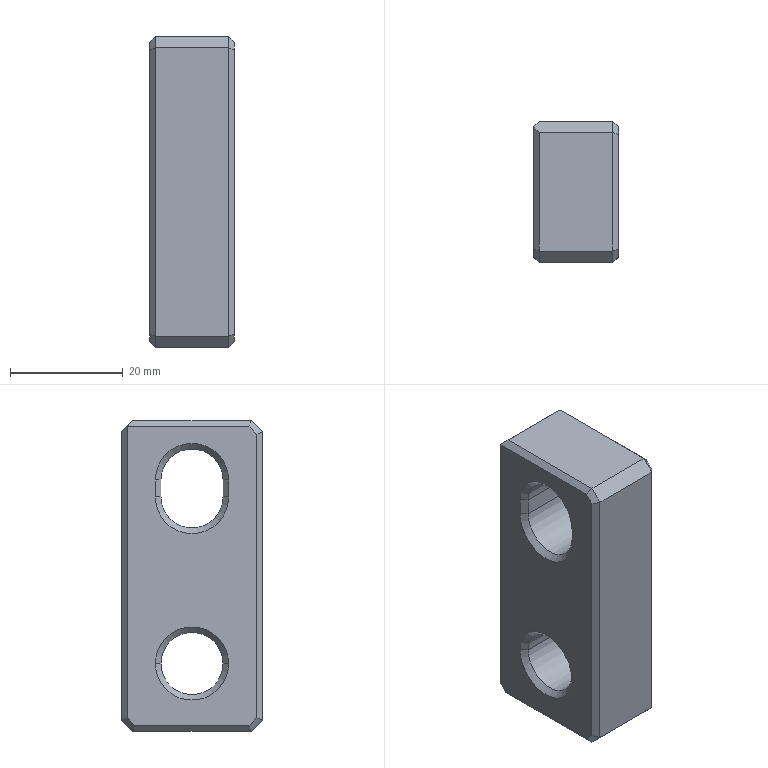Part | Creo | 1 solid | 43 faces | box 15 x 25 x 55 mm | volume 16927 mm3 | plane 31 | cone 8 | cylinder 4 | commonest cylinder face diameters 11 x4
STEP:
#1=CARTESIAN_POINT('',(0.,0.,0.));
#2=DIRECTION('',(0.,0.,1.));
#3=DIRECTION('',(1.,0.,0.));
#4=AXIS2_PLACEMENT_3D('',#1,#2,#3);
#5=CARTESIAN_POINT('',(-215.,-183.086,-24.));
#6=VERTEX_POINT('',#5);
#7=CARTESIAN_POINT('',(-215.,-162.914,-24.));
#8=VERTEX_POINT('',#7);
#9=CARTESIAN_POINT('',(-215.,-183.086,-24.));
#10=DIRECTION('',(0.,1.,0.));
#11=VECTOR('',#10,20.172);
#12=LINE('',#9,#11);
#13=EDGE_CURVE('',#6,#8,#12,.T.);
#14=ORIENTED_EDGE('',*,*,#13,.T.);
#15=CARTESIAN_POINT('',(-215.,-161.5,-22.586));
#16=VERTEX_POINT('',#15);
#17=CARTESIAN_POINT('',(-215.,-162.914,-24.));
#18=DIRECTION('',(0.,0.7071,0.7071));
#19=VECTOR('',#18,2.);
#20=LINE('',#17,#19);
#21=EDGE_CURVE('',#8,#16,#20,.T.);
#22=ORIENTED_EDGE('',*,*,#21,.T.);
#23=CARTESIAN_POINT('',(-215.,-161.5,29.));
#24=VERTEX_POINT('',#23);
#25=CARTESIAN_POINT('',(-215.,-161.5,-22.586));
#26=DIRECTION('',(0.,0.,1.));
#27=VECTOR('',#26,51.586);
#28=LINE('',#25,#27);
#29=EDGE_CURVE('',#16,#24,#28,.T.);
#30=ORIENTED_EDGE('',*,*,#29,.T.);
#31=CARTESIAN_POINT('',(-215.,-183.086,29.));
#32=VERTEX_POINT('',#31);
#33=CARTESIAN_POINT('',(-215.,-161.5,29.));
#34=DIRECTION('',(0.,-1.,0.));
#35=VECTOR('',#34,21.586);
#36=LINE('',#33,#35);
#37=EDGE_CURVE('',#24,#32,#36,.T.);
#38=ORIENTED_EDGE('',*,*,#37,.T.);
#39=CARTESIAN_POINT('',(-215.,-184.5,27.586));
#40=VERTEX_POINT('',#39);
#41=CARTESIAN_POINT('',(-215.,-183.086,29.));
#42=DIRECTION('',(0.,-0.7071,-0.7071));
#43=VECTOR('',#42,2.);
#44=LINE('',#41,#43);
#45=EDGE_CURVE('',#32,#40,#44,.T.);
#46=ORIENTED_EDGE('',*,*,#45,.T.);
#47=CARTESIAN_POINT('',(-215.,-184.5,-22.586));
#48=VERTEX_POINT('',#47);
#49=CARTESIAN_POINT('',(-215.,-184.5,27.586));
#50=DIRECTION('',(0.,0.,-1.));
#51=VECTOR('',#50,50.172);
#52=LINE('',#49,#51);
#53=EDGE_CURVE('',#40,#48,#52,.T.);
#54=ORIENTED_EDGE('',*,*,#53,.T.);
#55=CARTESIAN_POINT('',(-215.,-184.5,-22.586));
#56=DIRECTION('',(0.,0.7071,-0.7071));
#57=VECTOR('',#56,2.);
#58=LINE('',#55,#57);
#59=EDGE_CURVE('',#48,#6,#58,.T.);
#60=ORIENTED_EDGE('',*,*,#59,.T.);
#61=EDGE_LOOP('',(#14,#22,#30,#38,#46,#54,#60));
#62=FACE_OUTER_BOUND('',#61,.F.);
#63=CARTESIAN_POINT('',(-215.,-179.5,-13.));
#64=VERTEX_POINT('',#63);
#65=CARTESIAN_POINT('',(-215.,-166.5,-13.));
#66=VERTEX_POINT('',#65);
#67=CARTESIAN_POINT('',(-215.,-173.,-13.));
#68=DIRECTION('',(1.,0.,0.));
#69=DIRECTION('',(0.,-1.,0.));
#70=AXIS2_PLACEMENT_3D('',#67,#68,#69);
#71=CIRCLE('',#70,6.5);
#72=EDGE_CURVE('',#64,#66,#71,.T.);
#73=ORIENTED_EDGE('',*,*,#72,.F.);
#74=CARTESIAN_POINT('',(-215.,-173.,-13.));
#75=DIRECTION('',(1.,0.,0.));
#76=DIRECTION('',(0.,1.,0.));
#77=AXIS2_PLACEMENT_3D('',#74,#75,#76);
#78=CIRCLE('',#77,6.5);
#79=EDGE_CURVE('',#66,#64,#78,.T.);
#80=ORIENTED_EDGE('',*,*,#79,.F.);
#81=EDGE_LOOP('',(#73,#80));
#82=FACE_BOUND('',#81,.F.);
#83=CARTESIAN_POINT('',(-215.,-166.5,19.5));
#84=VERTEX_POINT('',#83);
#85=CARTESIAN_POINT('',(-215.,-179.5,19.5));
#86=VERTEX_POINT('',#85);
#87=CARTESIAN_POINT('',(-215.,-173.,19.5));
#88=DIRECTION('',(1.,0.,0.));
#89=DIRECTION('',(0.,1.,0.));
#90=AXIS2_PLACEMENT_3D('',#87,#88,#89);
#91=CIRCLE('',#90,6.5);
#92=EDGE_CURVE('',#84,#86,#91,.T.);
#93=ORIENTED_EDGE('',*,*,#92,.F.);
#94=CARTESIAN_POINT('',(-215.,-166.5,16.5));
#95=VERTEX_POINT('',#94);
#96=CARTESIAN_POINT('',(-215.,-166.5,19.5));
#97=DIRECTION('',(0.,0.,-1.));
#98=VECTOR('',#97,3.);
#99=LINE('',#96,#98);
#100=EDGE_CURVE('',#84,#95,#99,.T.);
#101=ORIENTED_EDGE('',*,*,#100,.T.);
#102=CARTESIAN_POINT('',(-215.,-179.5,16.5));
#103=VERTEX_POINT('',#102);
#104=CARTESIAN_POINT('',(-215.,-173.,16.5));
#105=DIRECTION('',(1.,0.,0.));
#106=DIRECTION('',(0.,-1.,0.));
#107=AXIS2_PLACEMENT_3D('',#104,#105,#106);
#108=CIRCLE('',#107,6.5);
#109=EDGE_CURVE('',#103,#95,#108,.T.);
#110=ORIENTED_EDGE('',*,*,#109,.F.);
#111=CARTESIAN_POINT('',(-215.,-179.5,16.5));
#112=DIRECTION('',(0.,0.,1.));
#113=VECTOR('',#112,3.);
#114=LINE('',#111,#113);
#115=EDGE_CURVE('',#103,#86,#114,.T.);
#116=ORIENTED_EDGE('',*,*,#115,.T.);
#117=EDGE_LOOP('',(#93,#101,#110,#116));
#118=FACE_BOUND('',#117,.F.);
#119=CARTESIAN_POINT('',(-215.,-160.5,30.));
#120=DIRECTION('',(-1.,0.,0.));
#121=DIRECTION('',(0.,-1.,0.));
#122=AXIS2_PLACEMENT_3D('',#119,#120,#121);
#123=PLANE('',#122);
#124=ADVANCED_FACE('',(#62,#82,#118),#123,.T.);
#125=CARTESIAN_POINT('',(-214.,-162.5,-25.));
#126=VERTEX_POINT('',#125);
#127=CARTESIAN_POINT('',(-214.,-162.5,-25.));
#128=DIRECTION('',(-0.6786,-0.2811,0.6786));
#129=VECTOR('',#128,1.474);
#130=LINE('',#127,#129);
#131=EDGE_CURVE('',#126,#8,#130,.T.);
#132=ORIENTED_EDGE('',*,*,#131,.T.);
#133=ORIENTED_EDGE('',*,*,#13,.F.);
#134=CARTESIAN_POINT('',(-214.,-183.5,-25.));
#135=VERTEX_POINT('',#134);
#136=CARTESIAN_POINT('',(-214.,-183.5,-25.));
#137=DIRECTION('',(-0.6786,0.2811,0.6786));
#138=VECTOR('',#137,1.474);
#139=LINE('',#136,#138);
#140=EDGE_CURVE('',#135,#6,#139,.T.);
#141=ORIENTED_EDGE('',*,*,#140,.F.);
#142=CARTESIAN_POINT('',(-214.,-162.5,-25.));
#143=DIRECTION('',(0.,-1.,0.));
#144=VECTOR('',#143,21.);
#145=LINE('',#142,#144);
#146=EDGE_CURVE('',#126,#135,#145,.T.);
#147=ORIENTED_EDGE('',*,*,#146,.F.);
#148=EDGE_LOOP('',(#132,#133,#141,#147));
#149=FACE_OUTER_BOUND('',#148,.F.);
#150=CARTESIAN_POINT('',(-215.,-160.5,-24.));
#151=DIRECTION('',(-0.7071,0.,-0.7071));
#152=DIRECTION('',(0.7071,0.,-0.7071));
#153=AXIS2_PLACEMENT_3D('',#150,#151,#152);
#154=PLANE('',#153);
#155=ADVANCED_FACE('',(#149),#154,.T.);
#156=CARTESIAN_POINT('',(-214.,-160.5,-23.));
#157=VERTEX_POINT('',#156);
#158=CARTESIAN_POINT('',(-214.,-160.5,-23.));
#159=DIRECTION('',(-0.6786,-0.6786,0.2811));
#160=VECTOR('',#159,1.474);
#161=LINE('',#158,#160);
#162=EDGE_CURVE('',#157,#16,#161,.T.);
#163=ORIENTED_EDGE('',*,*,#162,.T.);
#164=ORIENTED_EDGE('',*,*,#21,.F.);
#165=ORIENTED_EDGE('',*,*,#131,.F.);
#166=CARTESIAN_POINT('',(-214.,-160.5,-23.));
#167=DIRECTION('',(0.,-0.7071,-0.7071));
#168=VECTOR('',#167,2.828);
#169=LINE('',#166,#168);
#170=EDGE_CURVE('',#157,#126,#169,.T.);
#171=ORIENTED_EDGE('',*,*,#170,.F.);
#172=EDGE_LOOP('',(#163,#164,#165,#171));
#173=FACE_OUTER_BOUND('',#172,.F.);
#174=CARTESIAN_POINT('',(-215.,-134.707,4.207));
#175=DIRECTION('',(-0.7071,0.5,-0.5));
#176=DIRECTION('',(-0.5774,-0.8165,0.));
#177=AXIS2_PLACEMENT_3D('',#174,#175,#176);
#178=PLANE('',#177);
#179=ADVANCED_FACE('',(#173),#178,.T.);
#180=CARTESIAN_POINT('',(-214.,-160.5,28.));
#181=VERTEX_POINT('',#180);
#182=CARTESIAN_POINT('',(-215.,-161.5,29.));
#183=DIRECTION('',(0.5774,0.5774,-0.5774));
#184=VECTOR('',#183,1.732);
#185=LINE('',#182,#184);
#186=EDGE_CURVE('',#24,#181,#185,.T.);
#187=ORIENTED_EDGE('',*,*,#186,.F.);
#188=ORIENTED_EDGE('',*,*,#29,.F.);
#189=ORIENTED_EDGE('',*,*,#162,.F.);
#190=CARTESIAN_POINT('',(-214.,-160.5,28.));
#191=DIRECTION('',(0.,0.,-1.));
#192=VECTOR('',#191,51.);
#193=LINE('',#190,#192);
#194=EDGE_CURVE('',#181,#157,#193,.T.);
#195=ORIENTED_EDGE('',*,*,#194,.F.);
#196=EDGE_LOOP('',(#187,#188,#189,#195));
#197=FACE_OUTER_BOUND('',#196,.F.);
#198=CARTESIAN_POINT('',(-215.,-161.5,30.));
#199=DIRECTION('',(-0.7071,0.7071,0.));
#200=DIRECTION('',(-0.7071,-0.7071,0.));
#201=AXIS2_PLACEMENT_3D('',#198,#199,#200);
#202=PLANE('',#201);
#203=ADVANCED_FACE('',(#197),#202,.T.);
#204=CARTESIAN_POINT('',(-214.,-162.5,30.));
#205=VERTEX_POINT('',#204);
#206=CARTESIAN_POINT('',(-201.,-162.5,30.));
#207=VERTEX_POINT('',#206);
#208=CARTESIAN_POINT('',(-214.,-162.5,30.));
#209=DIRECTION('',(1.,0.,0.));
#210=VECTOR('',#209,13.);
#211=LINE('',#208,#210);
#212=EDGE_CURVE('',#205,#207,#211,.T.);
#213=ORIENTED_EDGE('',*,*,#212,.F.);
#214=CARTESIAN_POINT('',(-214.,-162.5,30.));
#215=DIRECTION('',(-0.5774,0.5774,-0.5774));
#216=VECTOR('',#215,1.732);
#217=LINE('',#214,#216);
#218=EDGE_CURVE('',#205,#24,#217,.T.);
#219=ORIENTED_EDGE('',*,*,#218,.T.);
#220=ORIENTED_EDGE('',*,*,#186,.T.);
#221=CARTESIAN_POINT('',(-201.,-160.5,28.));
#222=VERTEX_POINT('',#221);
#223=CARTESIAN_POINT('',(-201.,-160.5,28.));
#224=DIRECTION('',(-1.,0.,0.));
#225=VECTOR('',#224,13.);
#226=LINE('',#223,#225);
#227=EDGE_CURVE('',#222,#181,#226,.T.);
#228=ORIENTED_EDGE('',*,*,#227,.F.);
#229=CARTESIAN_POINT('',(-201.,-160.5,28.));
#230=DIRECTION('',(0.,-0.7071,0.7071));
#231=VECTOR('',#230,2.828);
#232=LINE('',#229,#231);
#233=EDGE_CURVE('',#222,#207,#232,.T.);
#234=ORIENTED_EDGE('',*,*,#233,.T.);
#235=EDGE_LOOP('',(#213,#219,#220,#228,#234));
#236=FACE_OUTER_BOUND('',#235,.F.);
#237=CARTESIAN_POINT('',(-215.,-160.5,28.));
#238=DIRECTION('',(0.,-0.7071,-0.7071));
#239=DIRECTION('',(0.,-0.7071,0.7071));
#240=AXIS2_PLACEMENT_3D('',#237,#238,#239);
#241=PLANE('',#240);
#242=ADVANCED_FACE('',(#236),#241,.F.);
#243=CARTESIAN_POINT('',(-201.,-183.5,30.));
#244=VERTEX_POINT('',#243);
#245=CARTESIAN_POINT('',(-214.,-183.5,30.));
#246=VERTEX_POINT('',#245);
#247=CARTESIAN_POINT('',(-201.,-183.5,30.));
#248=DIRECTION('',(-1.,0.,0.));
#249=VECTOR('',#248,13.);
#250=LINE('',#247,#249);
#251=EDGE_CURVE('',#244,#246,#250,.T.);
#252=ORIENTED_EDGE('',*,*,#251,.T.);
#253=CARTESIAN_POINT('',(-214.,-183.5,30.));
#254=DIRECTION('',(0.,1.,0.));
#255=VECTOR('',#254,21.);
#256=LINE('',#253,#255);
#257=EDGE_CURVE('',#246,#205,#256,.T.);
#258=ORIENTED_EDGE('',*,*,#257,.T.);
#259=ORIENTED_EDGE('',*,*,#212,.T.);
#260=CARTESIAN_POINT('',(-201.,-162.5,30.));
#261=DIRECTION('',(0.,-1.,0.));
#262=VECTOR('',#261,21.);
#263=LINE('',#260,#262);
#264=EDGE_CURVE('',#207,#244,#263,.T.);
#265=ORIENTED_EDGE('',*,*,#264,.T.);
#266=EDGE_LOOP('',(#252,#258,#259,#265));
#267=FACE_OUTER_BOUND('',#266,.F.);
#268=CARTESIAN_POINT('',(-215.,-185.5,30.));
#269=DIRECTION('',(0.,0.,-1.));
#270=DIRECTION('',(1.,0.,0.));
#271=AXIS2_PLACEMENT_3D('',#268,#269,#270);
#272=PLANE('',#271);
#273=ADVANCED_FACE('',(#267),#272,.F.);
#274=CARTESIAN_POINT('',(-214.,-185.5,28.));
#275=VERTEX_POINT('',#274);
#276=CARTESIAN_POINT('',(-201.,-185.5,28.));
#277=VERTEX_POINT('',#276);
#278=CARTESIAN_POINT('',(-214.,-185.5,28.));
#279=DIRECTION('',(1.,0.,0.));
#280=VECTOR('',#279,13.);
#281=LINE('',#278,#280);
#282=EDGE_CURVE('',#275,#277,#281,.T.);
#283=ORIENTED_EDGE('',*,*,#282,.F.);
#284=CARTESIAN_POINT('',(-214.,-185.5,28.));
#285=DIRECTION('',(0.,0.7071,0.7071));
#286=VECTOR('',#285,2.828);
#287=LINE('',#284,#286);
#288=EDGE_CURVE('',#275,#246,#287,.T.);
#289=ORIENTED_EDGE('',*,*,#288,.T.);
#290=ORIENTED_EDGE('',*,*,#251,.F.);
#291=CARTESIAN_POINT('',(-201.,-183.5,30.));
#292=DIRECTION('',(0.,-0.7071,-0.7071));
#293=VECTOR('',#292,2.828);
#294=LINE('',#291,#293);
#295=EDGE_CURVE('',#244,#277,#294,.T.);
#296=ORIENTED_EDGE('',*,*,#295,.T.);
#297=EDGE_LOOP('',(#283,#289,#290,#296));
#298=FACE_OUTER_BOUND('',#297,.F.);
#299=CARTESIAN_POINT('',(-215.,-183.5,30.));
#300=DIRECTION('',(0.,0.7071,-0.7071));
#301=DIRECTION('',(0.,-0.7071,-0.7071));
#302=AXIS2_PLACEMENT_3D('',#299,#300,#301);
#303=PLANE('',#302);
#304=ADVANCED_FACE('',(#298),#303,.F.);
#305=CARTESIAN_POINT('',(-201.,-185.5,-23.));
#306=VERTEX_POINT('',#305);
#307=CARTESIAN_POINT('',(-214.,-185.5,-23.));
#308=VERTEX_POINT('',#307);
#309=CARTESIAN_POINT('',(-201.,-185.5,-23.));
#310=DIRECTION('',(-1.,0.,0.));
#311=VECTOR('',#310,13.);
#312=LINE('',#309,#311);
#313=EDGE_CURVE('',#306,#308,#312,.T.);
#314=ORIENTED_EDGE('',*,*,#313,.T.);
#315=CARTESIAN_POINT('',(-214.,-185.5,-23.));
#316=DIRECTION('',(0.,0.,1.));
#317=VECTOR('',#316,51.);
#318=LINE('',#315,#317);
#319=EDGE_CURVE('',#308,#275,#318,.T.);
#320=ORIENTED_EDGE('',*,*,#319,.T.);
#321=ORIENTED_EDGE('',*,*,#282,.T.);
#322=CARTESIAN_POINT('',(-201.,-185.5,28.));
#323=DIRECTION('',(0.,0.,-1.));
#324=VECTOR('',#323,51.);
#325=LINE('',#322,#324);
#326=EDGE_CURVE('',#277,#306,#325,.T.);
#327=ORIENTED_EDGE('',*,*,#326,.T.);
#328=EDGE_LOOP('',(#314,#320,#321,#327));
#329=FACE_OUTER_BOUND('',#328,.F.);
#330=CARTESIAN_POINT('',(-215.,-185.5,-25.));
#331=DIRECTION('',(0.,1.,0.));
#332=DIRECTION('',(0.,0.,-1.));
#333=AXIS2_PLACEMENT_3D('',#330,#331,#332);
#334=PLANE('',#333);
#335=ADVANCED_FACE('',(#329),#334,.F.);
#336=CARTESIAN_POINT('',(-201.,-183.5,-25.));
#337=VERTEX_POINT('',#336);
#338=CARTESIAN_POINT('',(-214.,-183.5,-25.));
#339=DIRECTION('',(1.,0.,0.));
#340=VECTOR('',#339,13.);
#341=LINE('',#338,#340);
#342=EDGE_CURVE('',#135,#337,#341,.T.);
#343=ORIENTED_EDGE('',*,*,#342,.F.);
#344=CARTESIAN_POINT('',(-214.,-183.5,-25.));
#345=DIRECTION('',(0.,-0.7071,0.7071));
#346=VECTOR('',#345,2.828);
#347=LINE('',#344,#346);
#348=EDGE_CURVE('',#135,#308,#347,.T.);
#349=ORIENTED_EDGE('',*,*,#348,.T.);
#350=ORIENTED_EDGE('',*,*,#313,.F.);
#351=CARTESIAN_POINT('',(-201.,-185.5,-23.));
#352=DIRECTION('',(0.,0.7071,-0.7071));
#353=VECTOR('',#352,2.828);
#354=LINE('',#351,#353);
#355=EDGE_CURVE('',#306,#337,#354,.T.);
#356=ORIENTED_EDGE('',*,*,#355,.T.);
#357=EDGE_LOOP('',(#343,#349,#350,#356));
#358=FACE_OUTER_BOUND('',#357,.F.);
#359=CARTESIAN_POINT('',(-215.,-185.5,-23.));
#360=DIRECTION('',(0.,0.7071,0.7071));
#361=DIRECTION('',(0.,0.7071,-0.7071));
#362=AXIS2_PLACEMENT_3D('',#359,#360,#361);
#363=PLANE('',#362);
#364=ADVANCED_FACE('',(#358),#363,.F.);
#365=CARTESIAN_POINT('',(-201.,-162.5,-25.));
#366=VERTEX_POINT('',#365);
#367=CARTESIAN_POINT('',(-201.,-162.5,-25.));
#368=DIRECTION('',(-1.,0.,0.));
#369=VECTOR('',#368,13.);
#370=LINE('',#367,#369);
#371=EDGE_CURVE('',#366,#126,#370,.T.);
#372=ORIENTED_EDGE('',*,*,#371,.T.);
#373=ORIENTED_EDGE('',*,*,#146,.T.);
#374=ORIENTED_EDGE('',*,*,#342,.T.);
#375=CARTESIAN_POINT('',(-201.,-183.5,-25.));
#376=DIRECTION('',(0.,1.,0.));
#377=VECTOR('',#376,21.);
#378=LINE('',#375,#377);
#379=EDGE_CURVE('',#337,#366,#378,.T.);
#380=ORIENTED_EDGE('',*,*,#379,.T.);
#381=EDGE_LOOP('',(#372,#373,#374,#380));
#382=FACE_OUTER_BOUND('',#381,.F.);
#383=CARTESIAN_POINT('',(-215.,-160.5,-25.));
#384=DIRECTION('',(0.,0.,1.));
#385=DIRECTION('',(0.,1.,0.));
#386=AXIS2_PLACEMENT_3D('',#383,#384,#385);
#387=PLANE('',#386);
#388=ADVANCED_FACE('',(#382),#387,.F.);
#389=CARTESIAN_POINT('',(-201.,-160.5,-23.));
#390=VERTEX_POINT('',#389);
#391=CARTESIAN_POINT('',(-214.,-160.5,-23.));
#392=DIRECTION('',(1.,0.,0.));
#393=VECTOR('',#392,13.);
#394=LINE('',#391,#393);
#395=EDGE_CURVE('',#157,#390,#394,.T.);
#396=ORIENTED_EDGE('',*,*,#395,.F.);
#397=ORIENTED_EDGE('',*,*,#170,.T.);
#398=ORIENTED_EDGE('',*,*,#371,.F.);
#399=CARTESIAN_POINT('',(-201.,-162.5,-25.));
#400=DIRECTION('',(0.,0.7071,0.7071));
#401=VECTOR('',#400,2.828);
#402=LINE('',#399,#401);
#403=EDGE_CURVE('',#366,#390,#402,.T.);
#404=ORIENTED_EDGE('',*,*,#403,.T.);
#405=EDGE_LOOP('',(#396,#397,#398,#404));
#406=FACE_OUTER_BOUND('',#405,.F.);
#407=CARTESIAN_POINT('',(-215.,-162.5,-25.));
#408=DIRECTION('',(0.,-0.7071,0.7071));
#409=DIRECTION('',(0.,0.7071,0.7071));
#410=AXIS2_PLACEMENT_3D('',#407,#408,#409);
#411=PLANE('',#410);
#412=ADVANCED_FACE('',(#406),#411,.F.);
#413=ORIENTED_EDGE('',*,*,#227,.T.);
#414=ORIENTED_EDGE('',*,*,#194,.T.);
#415=ORIENTED_EDGE('',*,*,#395,.T.);
#416=CARTESIAN_POINT('',(-201.,-160.5,-23.));
#417=DIRECTION('',(0.,0.,1.));
#418=VECTOR('',#417,51.);
#419=LINE('',#416,#418);
#420=EDGE_CURVE('',#390,#222,#419,.T.);
#421=ORIENTED_EDGE('',*,*,#420,.T.);
#422=EDGE_LOOP('',(#413,#414,#415,#421));
#423=FACE_OUTER_BOUND('',#422,.F.);
#424=CARTESIAN_POINT('',(-215.,-160.5,30.));
#425=DIRECTION('',(0.,-1.,0.));
#426=DIRECTION('',(0.,0.,1.));
#427=AXIS2_PLACEMENT_3D('',#424,#425,#426);
#428=PLANE('',#427);
#429=ADVANCED_FACE('',(#423),#428,.F.);
#430=CARTESIAN_POINT('',(-200.,-161.5,27.586));
#431=VERTEX_POINT('',#430);
#432=CARTESIAN_POINT('',(-200.,-161.5,27.586));
#433=DIRECTION('',(-0.6786,0.6786,0.2811));
#434=VECTOR('',#433,1.474);
#435=LINE('',#432,#434);
#436=EDGE_CURVE('',#431,#222,#435,.T.);
#437=ORIENTED_EDGE('',*,*,#436,.T.);
#438=ORIENTED_EDGE('',*,*,#420,.F.);
#439=CARTESIAN_POINT('',(-200.,-161.5,-22.586));
#440=VERTEX_POINT('',#439);
#441=CARTESIAN_POINT('',(-200.,-161.5,-22.586));
#442=DIRECTION('',(-0.6786,0.6786,-0.2811));
#443=VECTOR('',#442,1.474);
#444=LINE('',#441,#443);
#445=EDGE_CURVE('',#440,#390,#444,.T.);
#446=ORIENTED_EDGE('',*,*,#445,.F.);
#447=CARTESIAN_POINT('',(-200.,-161.5,27.586));
#448=DIRECTION('',(0.,0.,-1.));
#449=VECTOR('',#448,50.172);
#450=LINE('',#447,#449);
#451=EDGE_CURVE('',#431,#440,#450,.T.);
#452=ORIENTED_EDGE('',*,*,#451,.F.);
#453=EDGE_LOOP('',(#437,#438,#446,#452));
#454=FACE_OUTER_BOUND('',#453,.F.);
#455=CARTESIAN_POINT('',(-201.,-160.5,30.));
#456=DIRECTION('',(-0.7071,-0.7071,0.));
#457=DIRECTION('',(0.7071,-0.7071,0.));
#458=AXIS2_PLACEMENT_3D('',#455,#456,#457);
#459=PLANE('',#458);
#460=ADVANCED_FACE('',(#454),#459,.F.);
#461=CARTESIAN_POINT('',(-200.,-162.914,29.));
#462=VERTEX_POINT('',#461);
#463=CARTESIAN_POINT('',(-200.,-162.914,29.));
#464=DIRECTION('',(-0.6786,0.2811,0.6786));
#465=VECTOR('',#464,1.474);
#466=LINE('',#463,#465);
#467=EDGE_CURVE('',#462,#207,#466,.T.);
#468=ORIENTED_EDGE('',*,*,#467,.T.);
#469=ORIENTED_EDGE('',*,*,#233,.F.);
#470=ORIENTED_EDGE('',*,*,#436,.F.);
#471=CARTESIAN_POINT('',(-200.,-162.914,29.));
#472=DIRECTION('',(0.,0.7071,-0.7071));
#473=VECTOR('',#472,2.);
#474=LINE('',#471,#473);
#475=EDGE_CURVE('',#462,#431,#474,.T.);
#476=ORIENTED_EDGE('',*,*,#475,.F.);
#477=EDGE_LOOP('',(#468,#469,#470,#476));
#478=FACE_OUTER_BOUND('',#477,.F.);
#479=CARTESIAN_POINT('',(-200.,-162.207,28.293));
#480=DIRECTION('',(-0.7071,-0.5,-0.5));
#481=DIRECTION('',(0.5774,-0.8165,0.));
#482=AXIS2_PLACEMENT_3D('',#479,#480,#481);
#483=PLANE('',#482);
#484=ADVANCED_FACE('',(#478),#483,.F.);
#485=CARTESIAN_POINT('',(-200.,-183.086,29.));
#486=VERTEX_POINT('',#485);
#487=CARTESIAN_POINT('',(-200.,-183.086,29.));
#488=DIRECTION('',(-0.6786,-0.2811,0.6786));
#489=VECTOR('',#488,1.474);
#490=LINE('',#487,#489);
#491=EDGE_CURVE('',#486,#244,#490,.T.);
#492=ORIENTED_EDGE('',*,*,#491,.T.);
#493=ORIENTED_EDGE('',*,*,#264,.F.);
#494=ORIENTED_EDGE('',*,*,#467,.F.);
#495=CARTESIAN_POINT('',(-200.,-183.086,29.));
#496=DIRECTION('',(0.,1.,0.));
#497=VECTOR('',#496,20.172);
#498=LINE('',#495,#497);
#499=EDGE_CURVE('',#486,#462,#498,.T.);
#500=ORIENTED_EDGE('',*,*,#499,.F.);
#501=EDGE_LOOP('',(#492,#493,#494,#500));
#502=FACE_OUTER_BOUND('',#501,.F.);
#503=CARTESIAN_POINT('',(-201.,-185.5,30.));
#504=DIRECTION('',(-0.7071,0.,-0.7071));
#505=DIRECTION('',(0.7071,0.,-0.7071));
#506=AXIS2_PLACEMENT_3D('',#503,#504,#505);
#507=PLANE('',#506);
#508=ADVANCED_FACE('',(#502),#507,.F.);
#509=ORIENTED_EDGE('',*,*,#491,.F.);
#510=CARTESIAN_POINT('',(-200.,-184.5,27.586));
#511=VERTEX_POINT('',#510);
#512=CARTESIAN_POINT('',(-200.,-184.5,27.586));
#513=DIRECTION('',(0.,0.7071,0.7071));
#514=VECTOR('',#513,2.);
#515=LINE('',#512,#514);
#516=EDGE_CURVE('',#511,#486,#515,.T.);
#517=ORIENTED_EDGE('',*,*,#516,.F.);
#518=CARTESIAN_POINT('',(-201.,-185.5,28.));
#519=DIRECTION('',(0.6786,0.6786,-0.2811));
#520=VECTOR('',#519,1.474);
#521=LINE('',#518,#520);
#522=EDGE_CURVE('',#277,#511,#521,.T.);
#523=ORIENTED_EDGE('',*,*,#522,.F.);
#524=ORIENTED_EDGE('',*,*,#295,.F.);
#525=EDGE_LOOP('',(#509,#517,#523,#524));
#526=FACE_OUTER_BOUND('',#525,.F.);
#527=CARTESIAN_POINT('',(-200.,-171.293,40.793));
#528=DIRECTION('',(-0.7071,0.5,-0.5));
#529=DIRECTION('',(0.5774,0.,-0.8165));
#530=AXIS2_PLACEMENT_3D('',#527,#528,#529);
#531=PLANE('',#530);
#532=ADVANCED_FACE('',(#526),#531,.F.);
#533=CARTESIAN_POINT('',(-200.,-162.914,-24.));
#534=VERTEX_POINT('',#533);
#535=CARTESIAN_POINT('',(-200.,-183.086,-24.));
#536=VERTEX_POINT('',#535);
#537=CARTESIAN_POINT('',(-200.,-162.914,-24.));
#538=DIRECTION('',(0.,-1.,0.));
#539=VECTOR('',#538,20.172);
#540=LINE('',#537,#539);
#541=EDGE_CURVE('',#534,#536,#540,.T.);
#542=ORIENTED_EDGE('',*,*,#541,.T.);
#543=CARTESIAN_POINT('',(-200.,-184.5,-22.586));
#544=VERTEX_POINT('',#543);
#545=CARTESIAN_POINT('',(-200.,-183.086,-24.));
#546=DIRECTION('',(0.,-0.7071,0.7071));
#547=VECTOR('',#546,2.);
#548=LINE('',#545,#547);
#549=EDGE_CURVE('',#536,#544,#548,.T.);
#550=ORIENTED_EDGE('',*,*,#549,.T.);
#551=CARTESIAN_POINT('',(-200.,-184.5,-22.586));
#552=DIRECTION('',(0.,0.,1.));
#553=VECTOR('',#552,50.172);
#554=LINE('',#551,#553);
#555=EDGE_CURVE('',#544,#511,#554,.T.);
#556=ORIENTED_EDGE('',*,*,#555,.T.);
#557=ORIENTED_EDGE('',*,*,#516,.T.);
#558=ORIENTED_EDGE('',*,*,#499,.T.);
#559=ORIENTED_EDGE('',*,*,#475,.T.);
#560=ORIENTED_EDGE('',*,*,#451,.T.);
#561=CARTESIAN_POINT('',(-200.,-161.5,-22.586));
#562=DIRECTION('',(0.,-0.7071,-0.7071));
#563=VECTOR('',#562,2.);
#564=LINE('',#561,#563);
#565=EDGE_CURVE('',#440,#534,#564,.T.);
#566=ORIENTED_EDGE('',*,*,#565,.T.);
#567=EDGE_LOOP('',(#542,#550,#556,#557,#558,#559,#560,#566));
#568=FACE_OUTER_BOUND('',#567,.F.);
#569=CARTESIAN_POINT('',(-200.,-179.5,19.5));
#570=VERTEX_POINT('',#569);
#571=CARTESIAN_POINT('',(-200.,-166.5,19.5));
#572=VERTEX_POINT('',#571);
#573=CARTESIAN_POINT('',(-200.,-173.,19.5));
#574=DIRECTION('',(-1.,0.,0.));
#575=DIRECTION('',(0.,-1.,0.));
#576=AXIS2_PLACEMENT_3D('',#573,#574,#575);
#577=CIRCLE('',#576,6.5);
#578=EDGE_CURVE('',#570,#572,#577,.T.);
#579=ORIENTED_EDGE('',*,*,#578,.F.);
#580=CARTESIAN_POINT('',(-200.,-179.5,16.5));
#581=VERTEX_POINT('',#580);
#582=CARTESIAN_POINT('',(-200.,-179.5,19.5));
#583=DIRECTION('',(0.,0.,-1.));
#584=VECTOR('',#583,3.);
#585=LINE('',#582,#584);
#586=EDGE_CURVE('',#570,#581,#585,.T.);
#587=ORIENTED_EDGE('',*,*,#586,.T.);
#588=CARTESIAN_POINT('',(-200.,-166.5,16.5));
#589=VERTEX_POINT('',#588);
#590=CARTESIAN_POINT('',(-200.,-173.,16.5));
#591=DIRECTION('',(-1.,0.,0.));
#592=DIRECTION('',(0.,1.,0.));
#593=AXIS2_PLACEMENT_3D('',#590,#591,#592);
#594=CIRCLE('',#593,6.5);
#595=EDGE_CURVE('',#589,#581,#594,.T.);
#596=ORIENTED_EDGE('',*,*,#595,.F.);
#597=CARTESIAN_POINT('',(-200.,-166.5,16.5));
#598=DIRECTION('',(0.,0.,1.));
#599=VECTOR('',#598,3.);
#600=LINE('',#597,#599);
#601=EDGE_CURVE('',#589,#572,#600,.T.);
#602=ORIENTED_EDGE('',*,*,#601,.T.);
#603=EDGE_LOOP('',(#579,#587,#596,#602));
#604=FACE_BOUND('',#603,.F.);
#605=CARTESIAN_POINT('',(-200.,-179.5,-13.));
#606=VERTEX_POINT('',#605);
#607=CARTESIAN_POINT('',(-200.,-166.5,-13.));
#608=VERTEX_POINT('',#607);
#609=CARTESIAN_POINT('',(-200.,-173.,-13.));
#610=DIRECTION('',(-1.,0.,0.));
#611=DIRECTION('',(0.,-1.,0.));
#612=AXIS2_PLACEMENT_3D('',#609,#610,#611);
#613=CIRCLE('',#612,6.5);
#614=EDGE_CURVE('',#606,#608,#613,.T.);
#615=ORIENTED_EDGE('',*,*,#614,.F.);
#616=CARTESIAN_POINT('',(-200.,-173.,-13.));
#617=DIRECTION('',(-1.,0.,0.));
#618=DIRECTION('',(0.,1.,0.));
#619=AXIS2_PLACEMENT_3D('',#616,#617,#618);
#620=CIRCLE('',#619,6.5);
#621=EDGE_CURVE('',#608,#606,#620,.T.);
#622=ORIENTED_EDGE('',*,*,#621,.F.);
#623=EDGE_LOOP('',(#615,#622));
#624=FACE_BOUND('',#623,.F.);
#625=CARTESIAN_POINT('',(-200.,-160.5,30.));
#626=DIRECTION('',(-1.,0.,0.));
#627=DIRECTION('',(0.,-1.,0.));
#628=AXIS2_PLACEMENT_3D('',#625,#626,#627);
#629=PLANE('',#628);
#630=ADVANCED_FACE('',(#568,#604,#624),#629,.F.);
#631=CARTESIAN_POINT('',(-201.,-183.5,-25.));
#632=DIRECTION('',(0.6786,0.2811,0.6786));
#633=VECTOR('',#632,1.474);
#634=LINE('',#631,#633);
#635=EDGE_CURVE('',#337,#536,#634,.T.);
#636=ORIENTED_EDGE('',*,*,#635,.T.);
#637=ORIENTED_EDGE('',*,*,#541,.F.);
#638=CARTESIAN_POINT('',(-201.,-162.5,-25.));
#639=DIRECTION('',(0.6786,-0.2811,0.6786));
#640=VECTOR('',#639,1.474);
#641=LINE('',#638,#640);
#642=EDGE_CURVE('',#366,#534,#641,.T.);
#643=ORIENTED_EDGE('',*,*,#642,.F.);
#644=ORIENTED_EDGE('',*,*,#379,.F.);
#645=EDGE_LOOP('',(#636,#637,#643,#644));
#646=FACE_OUTER_BOUND('',#645,.F.);
#647=CARTESIAN_POINT('',(-201.,-160.5,-25.));
#648=DIRECTION('',(-0.7071,0.,0.7071));
#649=DIRECTION('',(-0.7071,0.,-0.7071));
#650=AXIS2_PLACEMENT_3D('',#647,#648,#649);
#651=PLANE('',#650);
#652=ADVANCED_FACE('',(#646),#651,.F.);
#653=CARTESIAN_POINT('',(-201.,-185.5,-23.));
#654=DIRECTION('',(0.6786,0.6786,0.2811));
#655=VECTOR('',#654,1.474);
#656=LINE('',#653,#655);
#657=EDGE_CURVE('',#306,#544,#656,.T.);
#658=ORIENTED_EDGE('',*,*,#657,.T.);
#659=ORIENTED_EDGE('',*,*,#549,.F.);
#660=ORIENTED_EDGE('',*,*,#635,.F.);
#661=ORIENTED_EDGE('',*,*,#355,.F.);
#662=EDGE_LOOP('',(#658,#659,#660,#661));
#663=FACE_OUTER_BOUND('',#662,.F.);
#664=CARTESIAN_POINT('',(-200.,-198.793,-8.293));
#665=DIRECTION('',(-0.7071,0.5,0.5));
#666=DIRECTION('',(-0.5774,-0.8165,0.));
#667=AXIS2_PLACEMENT_3D('',#664,#665,#666);
#668=PLANE('',#667);
#669=ADVANCED_FACE('',(#663),#668,.F.);
#670=ORIENTED_EDGE('',*,*,#522,.T.);
#671=ORIENTED_EDGE('',*,*,#555,.F.);
#672=ORIENTED_EDGE('',*,*,#657,.F.);
#673=ORIENTED_EDGE('',*,*,#326,.F.);
#674=EDGE_LOOP('',(#670,#671,#672,#673));
#675=FACE_OUTER_BOUND('',#674,.F.);
#676=CARTESIAN_POINT('',(-201.,-185.5,-25.));
#677=DIRECTION('',(-0.7071,0.7071,0.));
#678=DIRECTION('',(-0.7071,-0.7071,0.));
#679=AXIS2_PLACEMENT_3D('',#676,#677,#678);
#680=PLANE('',#679);
#681=ADVANCED_FACE('',(#675),#680,.F.);
#682=ORIENTED_EDGE('',*,*,#642,.T.);
#683=ORIENTED_EDGE('',*,*,#565,.F.);
#684=ORIENTED_EDGE('',*,*,#445,.T.);
#685=ORIENTED_EDGE('',*,*,#403,.F.);
#686=EDGE_LOOP('',(#682,#683,#684,#685));
#687=FACE_OUTER_BOUND('',#686,.F.);
#688=CARTESIAN_POINT('',(-200.,-134.707,4.207));
#689=DIRECTION('',(-0.7071,-0.5,0.5));
#690=DIRECTION('',(0.5774,-0.8165,0.));
#691=AXIS2_PLACEMENT_3D('',#688,#689,#690);
#692=PLANE('',#691);
#693=ADVANCED_FACE('',(#687),#692,.F.);
#694=CARTESIAN_POINT('',(-201.,-178.5,19.5));
#695=VERTEX_POINT('',#694);
#696=CARTESIAN_POINT('',(-200.,-179.5,19.5));
#697=DIRECTION('',(-0.7071,0.7071,0.));
#698=VECTOR('',#697,1.414);
#699=LINE('',#696,#698);
#700=EDGE_CURVE('',#570,#695,#699,.T.);
#701=ORIENTED_EDGE('',*,*,#700,.F.);
#702=ORIENTED_EDGE('',*,*,#578,.T.);
#703=CARTESIAN_POINT('',(-201.,-167.5,19.5));
#704=VERTEX_POINT('',#703);
#705=CARTESIAN_POINT('',(-201.,-167.5,19.5));
#706=DIRECTION('',(0.7071,0.7071,0.));
#707=VECTOR('',#706,1.414);
#708=LINE('',#705,#707);
#709=EDGE_CURVE('',#704,#572,#708,.T.);
#710=ORIENTED_EDGE('',*,*,#709,.F.);
#711=CARTESIAN_POINT('',(-201.,-173.,19.5));
#712=DIRECTION('',(-1.,0.,0.));
#713=DIRECTION('',(0.,-1.,0.));
#714=AXIS2_PLACEMENT_3D('',#711,#712,#713);
#715=CIRCLE('',#714,5.5);
#716=EDGE_CURVE('',#695,#704,#715,.T.);
#717=ORIENTED_EDGE('',*,*,#716,.F.);
#718=EDGE_LOOP('',(#701,#702,#710,#717));
#719=FACE_OUTER_BOUND('',#718,.F.);
#720=CARTESIAN_POINT('',(-200.5,-173.,19.5));
#721=DIRECTION('',(1.,0.,0.));
#722=DIRECTION('',(0.,1.,0.));
#723=AXIS2_PLACEMENT_3D('',#720,#721,#722);
#724=CONICAL_SURFACE('',#723,6.,45.);
#725=ADVANCED_FACE('',(#719),#724,.F.);
#726=CARTESIAN_POINT('',(-201.,-178.5,16.5));
#727=VERTEX_POINT('',#726);
#728=CARTESIAN_POINT('',(-201.,-178.5,16.5));
#729=DIRECTION('',(0.7071,-0.7071,0.));
#730=VECTOR('',#729,1.414);
#731=LINE('',#728,#730);
#732=EDGE_CURVE('',#727,#581,#731,.T.);
#733=ORIENTED_EDGE('',*,*,#732,.T.);
#734=ORIENTED_EDGE('',*,*,#586,.F.);
#735=ORIENTED_EDGE('',*,*,#700,.T.);
#736=CARTESIAN_POINT('',(-201.,-178.5,16.5));
#737=DIRECTION('',(0.,0.,1.));
#738=VECTOR('',#737,3.);
#739=LINE('',#736,#738);
#740=EDGE_CURVE('',#727,#695,#739,.T.);
#741=ORIENTED_EDGE('',*,*,#740,.F.);
#742=EDGE_LOOP('',(#733,#734,#735,#741));
#743=FACE_OUTER_BOUND('',#742,.F.);
#744=CARTESIAN_POINT('',(-200.,-179.5,30.));
#745=DIRECTION('',(0.7071,0.7071,0.));
#746=DIRECTION('',(-0.7071,0.7071,0.));
#747=AXIS2_PLACEMENT_3D('',#744,#745,#746);
#748=PLANE('',#747);
#749=ADVANCED_FACE('',(#743),#748,.T.);
#750=ORIENTED_EDGE('',*,*,#732,.F.);
#751=CARTESIAN_POINT('',(-201.,-167.5,16.5));
#752=VERTEX_POINT('',#751);
#753=CARTESIAN_POINT('',(-201.,-173.,16.5));
#754=DIRECTION('',(-1.,0.,0.));
#755=DIRECTION('',(0.,1.,0.));
#756=AXIS2_PLACEMENT_3D('',#753,#754,#755);
#757=CIRCLE('',#756,5.5);
#758=EDGE_CURVE('',#752,#727,#757,.T.);
#759=ORIENTED_EDGE('',*,*,#758,.F.);
#760=CARTESIAN_POINT('',(-200.,-166.5,16.5));
#761=DIRECTION('',(-0.7071,-0.7071,0.));
#762=VECTOR('',#761,1.414);
#763=LINE('',#760,#762);
#764=EDGE_CURVE('',#589,#752,#763,.T.);
#765=ORIENTED_EDGE('',*,*,#764,.F.);
#766=ORIENTED_EDGE('',*,*,#595,.T.);
#767=EDGE_LOOP('',(#750,#759,#765,#766));
#768=FACE_OUTER_BOUND('',#767,.F.);
#769=CARTESIAN_POINT('',(-200.5,-173.,16.5));
#770=DIRECTION('',(1.,0.,0.));
#771=DIRECTION('',(0.,1.,0.));
#772=AXIS2_PLACEMENT_3D('',#769,#770,#771);
#773=CONICAL_SURFACE('',#772,6.,45.);
#774=ADVANCED_FACE('',(#768),#773,.F.);
#775=CARTESIAN_POINT('',(-214.,-178.5,16.5));
#776=VERTEX_POINT('',#775);
#777=CARTESIAN_POINT('',(-214.,-178.5,16.5));
#778=DIRECTION('',(1.,0.,0.));
#779=VECTOR('',#778,13.);
#780=LINE('',#777,#779);
#781=EDGE_CURVE('',#776,#727,#780,.T.);
#782=ORIENTED_EDGE('',*,*,#781,.F.);
#783=CARTESIAN_POINT('',(-214.,-167.5,16.5));
#784=VERTEX_POINT('',#783);
#785=CARTESIAN_POINT('',(-214.,-173.,16.5));
#786=DIRECTION('',(1.,0.,0.));
#787=DIRECTION('',(0.,-1.,0.));
#788=AXIS2_PLACEMENT_3D('',#785,#786,#787);
#789=CIRCLE('',#788,5.5);
#790=EDGE_CURVE('',#776,#784,#789,.T.);
#791=ORIENTED_EDGE('',*,*,#790,.T.);
#792=CARTESIAN_POINT('',(-201.,-167.5,16.5));
#793=DIRECTION('',(-1.,0.,0.));
#794=VECTOR('',#793,13.);
#795=LINE('',#792,#794);
#796=EDGE_CURVE('',#752,#784,#795,.T.);
#797=ORIENTED_EDGE('',*,*,#796,.F.);
#798=ORIENTED_EDGE('',*,*,#758,.T.);
#799=EDGE_LOOP('',(#782,#791,#797,#798));
#800=FACE_OUTER_BOUND('',#799,.F.);
#801=CARTESIAN_POINT('',(-215.,-173.,16.5));
#802=DIRECTION('',(1.,0.,0.));
#803=DIRECTION('',(0.,1.,0.));
#804=AXIS2_PLACEMENT_3D('',#801,#802,#803);
#805=CYLINDRICAL_SURFACE('',#804,5.5);
#806=ADVANCED_FACE('',(#800),#805,.F.);
#807=CARTESIAN_POINT('',(-214.,-178.5,19.5));
#808=VERTEX_POINT('',#807);
#809=CARTESIAN_POINT('',(-201.,-178.5,19.5));
#810=DIRECTION('',(-1.,0.,0.));
#811=VECTOR('',#810,13.);
#812=LINE('',#809,#811);
#813=EDGE_CURVE('',#695,#808,#812,.T.);
#814=ORIENTED_EDGE('',*,*,#813,.T.);
#815=CARTESIAN_POINT('',(-214.,-178.5,19.5));
#816=DIRECTION('',(0.,0.,-1.));
#817=VECTOR('',#816,3.);
#818=LINE('',#815,#817);
#819=EDGE_CURVE('',#808,#776,#818,.T.);
#820=ORIENTED_EDGE('',*,*,#819,.T.);
#821=ORIENTED_EDGE('',*,*,#781,.T.);
#822=ORIENTED_EDGE('',*,*,#740,.T.);
#823=EDGE_LOOP('',(#814,#820,#821,#822));
#824=FACE_OUTER_BOUND('',#823,.F.);
#825=CARTESIAN_POINT('',(-215.,-178.5,16.5));
#826=DIRECTION('',(0.,1.,0.));
#827=DIRECTION('',(0.,0.,-1.));
#828=AXIS2_PLACEMENT_3D('',#825,#826,#827);
#829=PLANE('',#828);
#830=ADVANCED_FACE('',(#824),#829,.T.);
#831=CARTESIAN_POINT('',(-214.,-167.5,19.5));
#832=VERTEX_POINT('',#831);
#833=CARTESIAN_POINT('',(-214.,-167.5,19.5));
#834=DIRECTION('',(1.,0.,0.));
#835=VECTOR('',#834,13.);
#836=LINE('',#833,#835);
#837=EDGE_CURVE('',#832,#704,#836,.T.);
#838=ORIENTED_EDGE('',*,*,#837,.F.);
#839=CARTESIAN_POINT('',(-214.,-173.,19.5));
#840=DIRECTION('',(1.,0.,0.));
#841=DIRECTION('',(0.,1.,0.));
#842=AXIS2_PLACEMENT_3D('',#839,#840,#841);
#843=CIRCLE('',#842,5.5);
#844=EDGE_CURVE('',#832,#808,#843,.T.);
#845=ORIENTED_EDGE('',*,*,#844,.T.);
#846=ORIENTED_EDGE('',*,*,#813,.F.);
#847=ORIENTED_EDGE('',*,*,#716,.T.);
#848=EDGE_LOOP('',(#838,#845,#846,#847));
#849=FACE_OUTER_BOUND('',#848,.F.);
#850=CARTESIAN_POINT('',(-215.,-173.,19.5));
#851=DIRECTION('',(1.,0.,0.));
#852=DIRECTION('',(0.,1.,0.));
#853=AXIS2_PLACEMENT_3D('',#850,#851,#852);
#854=CYLINDRICAL_SURFACE('',#853,5.5);
#855=ADVANCED_FACE('',(#849),#854,.F.);
#856=ORIENTED_EDGE('',*,*,#796,.T.);
#857=CARTESIAN_POINT('',(-214.,-167.5,16.5));
#858=DIRECTION('',(0.,0.,1.));
#859=VECTOR('',#858,3.);
#860=LINE('',#857,#859);
#861=EDGE_CURVE('',#784,#832,#860,.T.);
#862=ORIENTED_EDGE('',*,*,#861,.T.);
#863=ORIENTED_EDGE('',*,*,#837,.T.);
#864=CARTESIAN_POINT('',(-201.,-167.5,19.5));
#865=DIRECTION('',(0.,0.,-1.));
#866=VECTOR('',#865,3.);
#867=LINE('',#864,#866);
#868=EDGE_CURVE('',#704,#752,#867,.T.);
#869=ORIENTED_EDGE('',*,*,#868,.T.);
#870=EDGE_LOOP('',(#856,#862,#863,#869));
#871=FACE_OUTER_BOUND('',#870,.F.);
#872=CARTESIAN_POINT('',(-215.,-167.5,19.5));
#873=DIRECTION('',(0.,-1.,0.));
#874=DIRECTION('',(1.,0.,0.));
#875=AXIS2_PLACEMENT_3D('',#872,#873,#874);
#876=PLANE('',#875);
#877=ADVANCED_FACE('',(#871),#876,.T.);
#878=CARTESIAN_POINT('',(-215.,-166.5,19.5));
#879=DIRECTION('',(0.7071,-0.7071,0.));
#880=VECTOR('',#879,1.414);
#881=LINE('',#878,#880);
#882=EDGE_CURVE('',#84,#832,#881,.T.);
#883=ORIENTED_EDGE('',*,*,#882,.T.);
#884=ORIENTED_EDGE('',*,*,#861,.F.);
#885=CARTESIAN_POINT('',(-214.,-167.5,16.5));
#886=DIRECTION('',(-0.7071,0.7071,0.));
#887=VECTOR('',#886,1.414);
#888=LINE('',#885,#887);
#889=EDGE_CURVE('',#784,#95,#888,.T.);
#890=ORIENTED_EDGE('',*,*,#889,.T.);
#891=ORIENTED_EDGE('',*,*,#100,.F.);
#892=EDGE_LOOP('',(#883,#884,#890,#891));
#893=FACE_OUTER_BOUND('',#892,.F.);
#894=CARTESIAN_POINT('',(-214.,-167.5,19.5));
#895=DIRECTION('',(0.7071,0.7071,0.));
#896=DIRECTION('',(-0.7071,0.7071,0.));
#897=AXIS2_PLACEMENT_3D('',#894,#895,#896);
#898=PLANE('',#897);
#899=ADVANCED_FACE('',(#893),#898,.F.);
#900=ORIENTED_EDGE('',*,*,#882,.F.);
#901=ORIENTED_EDGE('',*,*,#92,.T.);
#902=CARTESIAN_POINT('',(-214.,-178.5,19.5));
#903=DIRECTION('',(-0.7071,-0.7071,0.));
#904=VECTOR('',#903,1.414);
#905=LINE('',#902,#904);
#906=EDGE_CURVE('',#808,#86,#905,.T.);
#907=ORIENTED_EDGE('',*,*,#906,.F.);
#908=ORIENTED_EDGE('',*,*,#844,.F.);
#909=EDGE_LOOP('',(#900,#901,#907,#908));
#910=FACE_OUTER_BOUND('',#909,.F.);
#911=CARTESIAN_POINT('',(-214.5,-173.,19.5));
#912=DIRECTION('',(-1.,0.,0.));
#913=DIRECTION('',(0.,-1.,0.));
#914=AXIS2_PLACEMENT_3D('',#911,#912,#913);
#915=CONICAL_SURFACE('',#914,6.,45.);
#916=ADVANCED_FACE('',(#910),#915,.F.);
#917=CARTESIAN_POINT('',(-215.,-179.5,16.5));
#918=DIRECTION('',(0.7071,0.7071,0.));
#919=VECTOR('',#918,1.414);
#920=LINE('',#917,#919);
#921=EDGE_CURVE('',#103,#776,#920,.T.);
#922=ORIENTED_EDGE('',*,*,#921,.T.);
#923=ORIENTED_EDGE('',*,*,#819,.F.);
#924=ORIENTED_EDGE('',*,*,#906,.T.);
#925=ORIENTED_EDGE('',*,*,#115,.F.);
#926=EDGE_LOOP('',(#922,#923,#924,#925));
#927=FACE_OUTER_BOUND('',#926,.F.);
#928=CARTESIAN_POINT('',(-214.,-178.5,16.5));
#929=DIRECTION('',(0.7071,-0.7071,0.));
#930=DIRECTION('',(0.7071,0.7071,0.));
#931=AXIS2_PLACEMENT_3D('',#928,#929,#930);
#932=PLANE('',#931);
#933=ADVANCED_FACE('',(#927),#932,.F.);
#934=ORIENTED_EDGE('',*,*,#889,.F.);
#935=ORIENTED_EDGE('',*,*,#790,.F.);
#936=ORIENTED_EDGE('',*,*,#921,.F.);
#937=ORIENTED_EDGE('',*,*,#109,.T.);
#938=EDGE_LOOP('',(#934,#935,#936,#937));
#939=FACE_OUTER_BOUND('',#938,.F.);
#940=CARTESIAN_POINT('',(-214.5,-173.,16.5));
#941=DIRECTION('',(-1.,0.,0.));
#942=DIRECTION('',(0.,-1.,0.));
#943=AXIS2_PLACEMENT_3D('',#940,#941,#942);
#944=CONICAL_SURFACE('',#943,6.,45.);
#945=ADVANCED_FACE('',(#939),#944,.F.);
#946=ORIENTED_EDGE('',*,*,#709,.T.);
#947=ORIENTED_EDGE('',*,*,#601,.F.);
#948=ORIENTED_EDGE('',*,*,#764,.T.);
#949=ORIENTED_EDGE('',*,*,#868,.F.);
#950=EDGE_LOOP('',(#946,#947,#948,#949));
#951=FACE_OUTER_BOUND('',#950,.F.);
#952=CARTESIAN_POINT('',(-200.,-166.5,30.));
#953=DIRECTION('',(0.7071,-0.7071,0.));
#954=DIRECTION('',(0.7071,0.7071,0.));
#955=AXIS2_PLACEMENT_3D('',#952,#953,#954);
#956=PLANE('',#955);
#957=ADVANCED_FACE('',(#951),#956,.T.);
#958=ORIENTED_EDGE('',*,*,#614,.T.);
#959=CARTESIAN_POINT('',(-201.,-167.5,-13.));
#960=VERTEX_POINT('',#959);
#961=CARTESIAN_POINT('',(-201.,-167.5,-13.));
#962=DIRECTION('',(0.7071,0.7071,0.));
#963=VECTOR('',#962,1.414);
#964=LINE('',#961,#963);
#965=EDGE_CURVE('',#960,#608,#964,.T.);
#966=ORIENTED_EDGE('',*,*,#965,.F.);
#967=CARTESIAN_POINT('',(-201.,-178.5,-13.));
#968=VERTEX_POINT('',#967);
#969=CARTESIAN_POINT('',(-201.,-173.,-13.));
#970=DIRECTION('',(-1.,0.,0.));
#971=DIRECTION('',(0.,-1.,0.));
#972=AXIS2_PLACEMENT_3D('',#969,#970,#971);
#973=CIRCLE('',#972,5.5);
#974=EDGE_CURVE('',#968,#960,#973,.T.);
#975=ORIENTED_EDGE('',*,*,#974,.F.);
#976=CARTESIAN_POINT('',(-201.,-178.5,-13.));
#977=DIRECTION('',(0.7071,-0.7071,0.));
#978=VECTOR('',#977,1.414);
#979=LINE('',#976,#978);
#980=EDGE_CURVE('',#968,#606,#979,.T.);
#981=ORIENTED_EDGE('',*,*,#980,.T.);
#982=EDGE_LOOP('',(#958,#966,#975,#981));
#983=FACE_OUTER_BOUND('',#982,.F.);
#984=CARTESIAN_POINT('',(-200.5,-173.,-13.));
#985=DIRECTION('',(1.,0.,0.));
#986=DIRECTION('',(0.,1.,0.));
#987=AXIS2_PLACEMENT_3D('',#984,#985,#986);
#988=CONICAL_SURFACE('',#987,6.,45.);
#989=ADVANCED_FACE('',(#983),#988,.F.);
#990=ORIENTED_EDGE('',*,*,#621,.T.);
#991=ORIENTED_EDGE('',*,*,#980,.F.);
#992=CARTESIAN_POINT('',(-201.,-173.,-13.));
#993=DIRECTION('',(-1.,0.,0.));
#994=DIRECTION('',(0.,1.,0.));
#995=AXIS2_PLACEMENT_3D('',#992,#993,#994);
#996=CIRCLE('',#995,5.5);
#997=EDGE_CURVE('',#960,#968,#996,.T.);
#998=ORIENTED_EDGE('',*,*,#997,.F.);
#999=ORIENTED_EDGE('',*,*,#965,.T.);
#1000=EDGE_LOOP('',(#990,#991,#998,#999));
#1001=FACE_OUTER_BOUND('',#1000,.F.);
#1002=CARTESIAN_POINT('',(-200.5,-173.,-13.));
#1003=DIRECTION('',(1.,0.,0.));
#1004=DIRECTION('',(0.,1.,0.));
#1005=AXIS2_PLACEMENT_3D('',#1002,#1003,#1004);
#1006=CONICAL_SURFACE('',#1005,6.,45.);
#1007=ADVANCED_FACE('',(#1001),#1006,.F.);
#1008=ORIENTED_EDGE('',*,*,#997,.T.);
#1009=CARTESIAN_POINT('',(-214.,-178.5,-13.));
#1010=VERTEX_POINT('',#1009);
#1011=CARTESIAN_POINT('',(-214.,-178.5,-13.));
#1012=DIRECTION('',(1.,0.,0.));
#1013=VECTOR('',#1012,13.);
#1014=LINE('',#1011,#1013);
#1015=EDGE_CURVE('',#1010,#968,#1014,.T.);
#1016=ORIENTED_EDGE('',*,*,#1015,.F.);
#1017=CARTESIAN_POINT('',(-214.,-167.5,-13.));
#1018=VERTEX_POINT('',#1017);
#1019=CARTESIAN_POINT('',(-214.,-173.,-13.));
#1020=DIRECTION('',(1.,0.,0.));
#1021=DIRECTION('',(0.,-1.,0.));
#1022=AXIS2_PLACEMENT_3D('',#1019,#1020,#1021);
#1023=CIRCLE('',#1022,5.5);
#1024=EDGE_CURVE('',#1010,#1018,#1023,.T.);
#1025=ORIENTED_EDGE('',*,*,#1024,.T.);
#1026=CARTESIAN_POINT('',(-214.,-167.5,-13.));
#1027=DIRECTION('',(1.,0.,0.));
#1028=VECTOR('',#1027,13.);
#1029=LINE('',#1026,#1028);
#1030=EDGE_CURVE('',#1018,#960,#1029,.T.);
#1031=ORIENTED_EDGE('',*,*,#1030,.T.);
#1032=EDGE_LOOP('',(#1008,#1016,#1025,#1031));
#1033=FACE_OUTER_BOUND('',#1032,.F.);
#1034=CARTESIAN_POINT('',(-215.,-173.,-13.));
#1035=DIRECTION('',(1.,0.,0.));
#1036=DIRECTION('',(0.,1.,0.));
#1037=AXIS2_PLACEMENT_3D('',#1034,#1035,#1036);
#1038=CYLINDRICAL_SURFACE('',#1037,5.5);
#1039=ADVANCED_FACE('',(#1033),#1038,.F.);
#1040=ORIENTED_EDGE('',*,*,#974,.T.);
#1041=ORIENTED_EDGE('',*,*,#1030,.F.);
#1042=CARTESIAN_POINT('',(-214.,-173.,-13.));
#1043=DIRECTION('',(1.,0.,0.));
#1044=DIRECTION('',(0.,1.,0.));
#1045=AXIS2_PLACEMENT_3D('',#1042,#1043,#1044);
#1046=CIRCLE('',#1045,5.5);
#1047=EDGE_CURVE('',#1018,#1010,#1046,.T.);
#1048=ORIENTED_EDGE('',*,*,#1047,.T.);
#1049=ORIENTED_EDGE('',*,*,#1015,.T.);
#1050=EDGE_LOOP('',(#1040,#1041,#1048,#1049));
#1051=FACE_OUTER_BOUND('',#1050,.F.);
#1052=CARTESIAN_POINT('',(-215.,-173.,-13.));
#1053=DIRECTION('',(1.,0.,0.));
#1054=DIRECTION('',(0.,1.,0.));
#1055=AXIS2_PLACEMENT_3D('',#1052,#1053,#1054);
#1056=CYLINDRICAL_SURFACE('',#1055,5.5);
#1057=ADVANCED_FACE('',(#1051),#1056,.F.);
#1058=ORIENTED_EDGE('',*,*,#1047,.F.);
#1059=CARTESIAN_POINT('',(-214.,-167.5,-13.));
#1060=DIRECTION('',(-0.7071,0.7071,0.));
#1061=VECTOR('',#1060,1.414);
#1062=LINE('',#1059,#1061);
#1063=EDGE_CURVE('',#1018,#66,#1062,.T.);
#1064=ORIENTED_EDGE('',*,*,#1063,.T.);
#1065=ORIENTED_EDGE('',*,*,#79,.T.);
#1066=CARTESIAN_POINT('',(-214.,-178.5,-13.));
#1067=DIRECTION('',(-0.7071,-0.7071,0.));
#1068=VECTOR('',#1067,1.414);
#1069=LINE('',#1066,#1068);
#1070=EDGE_CURVE('',#1010,#64,#1069,.T.);
#1071=ORIENTED_EDGE('',*,*,#1070,.F.);
#1072=EDGE_LOOP('',(#1058,#1064,#1065,#1071));
#1073=FACE_OUTER_BOUND('',#1072,.F.);
#1074=CARTESIAN_POINT('',(-214.5,-173.,-13.));
#1075=DIRECTION('',(-1.,0.,0.));
#1076=DIRECTION('',(0.,-1.,0.));
#1077=AXIS2_PLACEMENT_3D('',#1074,#1075,#1076);
#1078=CONICAL_SURFACE('',#1077,6.,45.);
#1079=ADVANCED_FACE('',(#1073),#1078,.F.);
#1080=ORIENTED_EDGE('',*,*,#1024,.F.);
#1081=ORIENTED_EDGE('',*,*,#1070,.T.);
#1082=ORIENTED_EDGE('',*,*,#72,.T.);
#1083=ORIENTED_EDGE('',*,*,#1063,.F.);
#1084=EDGE_LOOP('',(#1080,#1081,#1082,#1083));
#1085=FACE_OUTER_BOUND('',#1084,.F.);
#1086=CARTESIAN_POINT('',(-214.5,-173.,-13.));
#1087=DIRECTION('',(-1.,0.,0.));
#1088=DIRECTION('',(0.,-1.,0.));
#1089=AXIS2_PLACEMENT_3D('',#1086,#1087,#1088);
#1090=CONICAL_SURFACE('',#1089,6.,45.);
#1091=ADVANCED_FACE('',(#1085),#1090,.F.);
#1092=ORIENTED_EDGE('',*,*,#140,.T.);
#1093=ORIENTED_EDGE('',*,*,#59,.F.);
#1094=CARTESIAN_POINT('',(-215.,-184.5,-22.586));
#1095=DIRECTION('',(0.6786,-0.6786,-0.2811));
#1096=VECTOR('',#1095,1.474);
#1097=LINE('',#1094,#1096);
#1098=EDGE_CURVE('',#48,#308,#1097,.T.);
#1099=ORIENTED_EDGE('',*,*,#1098,.T.);
#1100=ORIENTED_EDGE('',*,*,#348,.F.);
#1101=EDGE_LOOP('',(#1092,#1093,#1099,#1100));
#1102=FACE_OUTER_BOUND('',#1101,.F.);
#1103=CARTESIAN_POINT('',(-215.,-198.793,-8.293));
#1104=DIRECTION('',(-0.7071,-0.5,-0.5));
#1105=DIRECTION('',(0.5774,-0.8165,0.));
#1106=AXIS2_PLACEMENT_3D('',#1103,#1104,#1105);
#1107=PLANE('',#1106);
#1108=ADVANCED_FACE('',(#1102),#1107,.T.);
#1109=CARTESIAN_POINT('',(-215.,-184.5,27.586));
#1110=DIRECTION('',(0.6786,-0.6786,0.2811));
#1111=VECTOR('',#1110,1.474);
#1112=LINE('',#1109,#1111);
#1113=EDGE_CURVE('',#40,#275,#1112,.T.);
#1114=ORIENTED_EDGE('',*,*,#1113,.T.);
#1115=ORIENTED_EDGE('',*,*,#319,.F.);
#1116=ORIENTED_EDGE('',*,*,#1098,.F.);
#1117=ORIENTED_EDGE('',*,*,#53,.F.);
#1118=EDGE_LOOP('',(#1114,#1115,#1116,#1117));
#1119=FACE_OUTER_BOUND('',#1118,.F.);
#1120=CARTESIAN_POINT('',(-215.,-184.5,30.));
#1121=DIRECTION('',(-0.7071,-0.7071,0.));
#1122=DIRECTION('',(0.7071,-0.7071,0.));
#1123=AXIS2_PLACEMENT_3D('',#1120,#1121,#1122);
#1124=PLANE('',#1123);
#1125=ADVANCED_FACE('',(#1119),#1124,.T.);
#1126=CARTESIAN_POINT('',(-215.,-183.086,29.));
#1127=DIRECTION('',(0.6786,-0.2811,0.6786));
#1128=VECTOR('',#1127,1.474);
#1129=LINE('',#1126,#1128);
#1130=EDGE_CURVE('',#32,#246,#1129,.T.);
#1131=ORIENTED_EDGE('',*,*,#1130,.T.);
#1132=ORIENTED_EDGE('',*,*,#288,.F.);
#1133=ORIENTED_EDGE('',*,*,#1113,.F.);
#1134=ORIENTED_EDGE('',*,*,#45,.F.);
#1135=EDGE_LOOP('',(#1131,#1132,#1133,#1134));
#1136=FACE_OUTER_BOUND('',#1135,.F.);
#1137=CARTESIAN_POINT('',(-215.,-171.293,40.793));
#1138=DIRECTION('',(-0.7071,-0.5,0.5));
#1139=DIRECTION('',(-0.5774,0.,-0.8165));
#1140=AXIS2_PLACEMENT_3D('',#1137,#1138,#1139);
#1141=PLANE('',#1140);
#1142=ADVANCED_FACE('',(#1136),#1141,.T.);
#1143=ORIENTED_EDGE('',*,*,#218,.F.);
#1144=ORIENTED_EDGE('',*,*,#257,.F.);
#1145=ORIENTED_EDGE('',*,*,#1130,.F.);
#1146=ORIENTED_EDGE('',*,*,#37,.F.);
#1147=EDGE_LOOP('',(#1143,#1144,#1145,#1146));
#1148=FACE_OUTER_BOUND('',#1147,.F.);
#1149=CARTESIAN_POINT('',(-215.,-160.5,29.));
#1150=DIRECTION('',(-0.7071,0.,0.7071));
#1151=DIRECTION('',(-0.7071,0.,-0.7071));
#1152=AXIS2_PLACEMENT_3D('',#1149,#1150,#1151);
#1153=PLANE('',#1152);
#1154=ADVANCED_FACE('',(#1148),#1153,.T.);
#1155=CLOSED_SHELL('',(#124,#155,#179,#203,#242,#273,#304,#335,#364,#388,#412,#429,#460,#484,#508,#532,#630,#652,#669,#681,#693,#725,#749,#774,#806,#830,#855,#877,#899,#916,#933,#945,#957,#989,#1007,#1039,#1057,#1079,#1091,#1108,#1125,#1142,#1154));
#1156=MANIFOLD_SOLID_BREP('',#1155);
#1157=(LENGTH_UNIT()NAMED_UNIT(*)SI_UNIT(.MILLI.,.METRE.));
#1158=UNCERTAINTY_MEASURE_WITH_UNIT(LENGTH_MEASURE(0.006281),#1157,'','');
#1159=(NAMED_UNIT(*)PLANE_ANGLE_UNIT()SI_UNIT($,.RADIAN.));
#1160=PLANE_ANGLE_MEASURE_WITH_UNIT(PLANE_ANGLE_MEASURE(0.01745),#1159);
#1161=(CONVERSION_BASED_UNIT('DEGREE',#1160)NAMED_UNIT(*)PLANE_ANGLE_UNIT());
#1162=(NAMED_UNIT(*)SI_UNIT($,.STERADIAN.)SOLID_ANGLE_UNIT());
#1163=(GEOMETRIC_REPRESENTATION_CONTEXT(3)GLOBAL_UNCERTAINTY_ASSIGNED_CONTEXT((#1158))GLOBAL_UNIT_ASSIGNED_CONTEXT((#1157,#1161,#1162))REPRESENTATION_CONTEXT('',''));
#1164=ADVANCED_BREP_SHAPE_REPRESENTATION('',(#4,#1156),#1163);